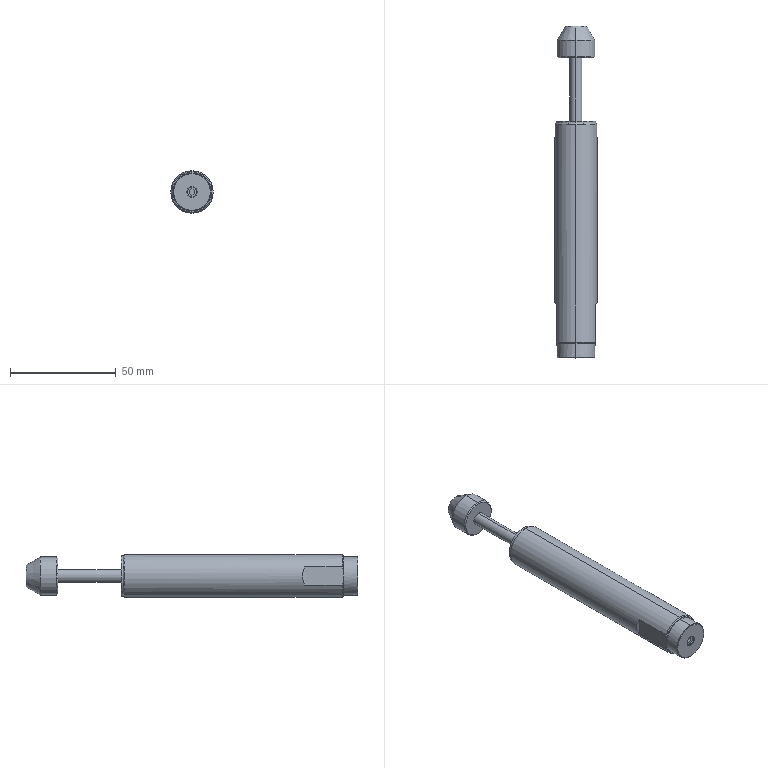Part | SolidWorks | features BaseBody 1 | 1 solid | 46 faces | box 20 x 157 x 20 mm | volume 38514 mm3 | plane 19 | cone 15 | cylinder 12 | commonest cylinder face diameters 18 x4 4.459 x2 6 x2 19 x2 20 x2
STEP:
#1=CARTESIAN_POINT('',(0.,0.2705,2.23));
#2=VERTEX_POINT('',#1);
#3=CARTESIAN_POINT('',(0.,0.2705,-2.23));
#4=VERTEX_POINT('',#3);
#5=CARTESIAN_POINT('',(0.,0.2705,0.));
#6=DIRECTION('',(0.,-1.,0.));
#7=DIRECTION('',(0.,0.,-1.));
#8=AXIS2_PLACEMENT_3D('',#5,#6,#7);
#9=CIRCLE('',#8,2.23);
#10=EDGE_CURVE('',#2,#4,#9,.T.);
#11=ORIENTED_EDGE('',*,*,#10,.F.);
#12=CARTESIAN_POINT('',(0.,0.,2.5));
#13=VERTEX_POINT('',#12);
#14=CARTESIAN_POINT('',(0.,0.2705,2.23));
#15=DIRECTION('',(0.,-0.7071,0.7071));
#16=VECTOR('',#15,1000.);
#17=LINE('',#14,#16);
#18=EDGE_CURVE('',#2,#13,#17,.T.);
#19=ORIENTED_EDGE('',*,*,#18,.T.);
#20=CARTESIAN_POINT('',(0.,0.,-2.5));
#21=VERTEX_POINT('',#20);
#22=CARTESIAN_POINT('',(0.,0.,0.));
#23=DIRECTION('',(0.,-1.,0.));
#24=DIRECTION('',(0.,0.,-1.));
#25=AXIS2_PLACEMENT_3D('',#22,#23,#24);
#26=CIRCLE('',#25,2.5);
#27=EDGE_CURVE('',#13,#21,#26,.T.);
#28=ORIENTED_EDGE('',*,*,#27,.T.);
#29=CARTESIAN_POINT('',(0.,0.2705,-2.23));
#30=DIRECTION('',(0.,-0.7071,-0.7071));
#31=VECTOR('',#30,1000.);
#32=LINE('',#29,#31);
#33=EDGE_CURVE('',#4,#21,#32,.T.);
#34=ORIENTED_EDGE('',*,*,#33,.F.);
#35=EDGE_LOOP('',(#11,#19,#28,#34));
#36=FACE_OUTER_BOUND('',#35,.T.);
#37=CARTESIAN_POINT('',(0.,0.2705,0.));
#38=DIRECTION('',(0.,-1.,0.));
#39=DIRECTION('',(0.,0.,-1.));
#40=AXIS2_PLACEMENT_3D('',#37,#38,#39);
#41=CONICAL_SURFACE('',#40,2.23,0.7854);
#42=ADVANCED_FACE('',(#36),#41,.F.);
#43=CARTESIAN_POINT('',(0.,0.2705,0.));
#44=DIRECTION('',(0.,-1.,0.));
#45=DIRECTION('',(0.,0.,-1.));
#46=AXIS2_PLACEMENT_3D('',#43,#44,#45);
#47=CIRCLE('',#46,2.23);
#48=EDGE_CURVE('',#4,#2,#47,.T.);
#49=ORIENTED_EDGE('',*,*,#48,.T.);
#50=CARTESIAN_POINT('',(0.,0.9295,2.23));
#51=VERTEX_POINT('',#50);
#52=CARTESIAN_POINT('',(0.,0.,2.23));
#53=DIRECTION('',(0.,1.,0.));
#54=VECTOR('',#53,1000.);
#55=LINE('',#52,#54);
#56=EDGE_CURVE('',#2,#51,#55,.T.);
#57=ORIENTED_EDGE('',*,*,#56,.T.);
#58=CARTESIAN_POINT('',(0.,0.9295,-2.23));
#59=VERTEX_POINT('',#58);
#60=CARTESIAN_POINT('',(0.,0.9295,0.));
#61=DIRECTION('',(0.,-1.,0.));
#62=DIRECTION('',(0.,0.,-1.));
#63=AXIS2_PLACEMENT_3D('',#60,#61,#62);
#64=CIRCLE('',#63,2.23);
#65=EDGE_CURVE('',#59,#51,#64,.T.);
#66=ORIENTED_EDGE('',*,*,#65,.F.);
#67=CARTESIAN_POINT('',(0.,0.,-2.23));
#68=DIRECTION('',(0.,1.,0.));
#69=VECTOR('',#68,1000.);
#70=LINE('',#67,#69);
#71=EDGE_CURVE('',#4,#59,#70,.T.);
#72=ORIENTED_EDGE('',*,*,#71,.F.);
#73=EDGE_LOOP('',(#49,#57,#66,#72));
#74=FACE_OUTER_BOUND('',#73,.T.);
#75=CARTESIAN_POINT('',(0.,0.,0.));
#76=DIRECTION('',(0.,1.,0.));
#77=DIRECTION('',(0.,0.,-1.));
#78=AXIS2_PLACEMENT_3D('',#75,#76,#77);
#79=CYLINDRICAL_SURFACE('',#78,2.23);
#80=ADVANCED_FACE('',(#74),#79,.F.);
#81=CARTESIAN_POINT('',(0.,0.9295,0.));
#82=DIRECTION('',(0.,-1.,0.));
#83=DIRECTION('',(0.,0.,-1.));
#84=AXIS2_PLACEMENT_3D('',#81,#82,#83);
#85=CIRCLE('',#84,2.23);
#86=EDGE_CURVE('',#51,#59,#85,.T.);
#87=ORIENTED_EDGE('',*,*,#86,.T.);
#88=CARTESIAN_POINT('',(0.,1.2,-2.5));
#89=VERTEX_POINT('',#88);
#90=CARTESIAN_POINT('',(0.,1.2,-2.5));
#91=DIRECTION('',(0.,0.7071,-0.7071));
#92=VECTOR('',#91,1000.);
#93=LINE('',#90,#92);
#94=EDGE_CURVE('',#59,#89,#93,.T.);
#95=ORIENTED_EDGE('',*,*,#94,.T.);
#96=CARTESIAN_POINT('',(0.,1.2,2.5));
#97=VERTEX_POINT('',#96);
#98=CARTESIAN_POINT('',(0.,1.2,0.));
#99=DIRECTION('',(0.,-1.,0.));
#100=DIRECTION('',(0.,0.,-1.));
#101=AXIS2_PLACEMENT_3D('',#98,#99,#100);
#102=CIRCLE('',#101,2.5);
#103=EDGE_CURVE('',#97,#89,#102,.T.);
#104=ORIENTED_EDGE('',*,*,#103,.F.);
#105=CARTESIAN_POINT('',(0.,1.2,2.5));
#106=DIRECTION('',(0.,0.7071,0.7071));
#107=VECTOR('',#106,1000.);
#108=LINE('',#105,#107);
#109=EDGE_CURVE('',#51,#97,#108,.T.);
#110=ORIENTED_EDGE('',*,*,#109,.F.);
#111=EDGE_LOOP('',(#87,#95,#104,#110));
#112=FACE_OUTER_BOUND('',#111,.T.);
#113=CARTESIAN_POINT('',(0.,1.2,0.));
#114=DIRECTION('',(0.,1.,0.));
#115=DIRECTION('',(0.,0.,1.));
#116=AXIS2_PLACEMENT_3D('',#113,#114,#115);
#117=CONICAL_SURFACE('',#116,2.5,0.7854);
#118=ADVANCED_FACE('',(#112),#117,.F.);
#119=CARTESIAN_POINT('',(0.,0.,-8.7));
#120=VERTEX_POINT('',#119);
#121=CARTESIAN_POINT('',(0.,0.,8.7));
#122=VERTEX_POINT('',#121);
#123=CARTESIAN_POINT('',(0.,0.,0.));
#124=DIRECTION('',(0.,-1.,0.));
#125=DIRECTION('',(0.,0.,-1.));
#126=AXIS2_PLACEMENT_3D('',#123,#124,#125);
#127=CIRCLE('',#126,8.7);
#128=EDGE_CURVE('',#120,#122,#127,.T.);
#129=ORIENTED_EDGE('',*,*,#128,.F.);
#130=CARTESIAN_POINT('',(0.,0.3,-9.));
#131=VERTEX_POINT('',#130);
#132=CARTESIAN_POINT('',(0.,0.3,-9.));
#133=DIRECTION('',(0.,0.7071,-0.7071));
#134=VECTOR('',#133,1000.);
#135=LINE('',#132,#134);
#136=EDGE_CURVE('',#120,#131,#135,.T.);
#137=ORIENTED_EDGE('',*,*,#136,.T.);
#138=CARTESIAN_POINT('',(0.,0.3,9.));
#139=VERTEX_POINT('',#138);
#140=CARTESIAN_POINT('',(0.,0.3,0.));
#141=DIRECTION('',(0.,-1.,0.));
#142=DIRECTION('',(0.,0.,-1.));
#143=AXIS2_PLACEMENT_3D('',#140,#141,#142);
#144=CIRCLE('',#143,9.);
#145=EDGE_CURVE('',#131,#139,#144,.T.);
#146=ORIENTED_EDGE('',*,*,#145,.T.);
#147=CARTESIAN_POINT('',(0.,0.3,9.));
#148=DIRECTION('',(0.,0.7071,0.7071));
#149=VECTOR('',#148,1000.);
#150=LINE('',#147,#149);
#151=EDGE_CURVE('',#122,#139,#150,.T.);
#152=ORIENTED_EDGE('',*,*,#151,.F.);
#153=EDGE_LOOP('',(#129,#137,#146,#152));
#154=FACE_OUTER_BOUND('',#153,.T.);
#155=CARTESIAN_POINT('',(0.,0.3,0.));
#156=DIRECTION('',(0.,1.,0.));
#157=DIRECTION('',(0.,0.,1.));
#158=AXIS2_PLACEMENT_3D('',#155,#156,#157);
#159=CONICAL_SURFACE('',#158,9.,0.7854);
#160=ADVANCED_FACE('',(#154),#159,.T.);
#161=CARTESIAN_POINT('',(0.,0.3,0.));
#162=DIRECTION('',(0.,-1.,0.));
#163=DIRECTION('',(0.,0.,-1.));
#164=AXIS2_PLACEMENT_3D('',#161,#162,#163);
#165=CIRCLE('',#164,9.);
#166=EDGE_CURVE('',#139,#131,#165,.T.);
#167=ORIENTED_EDGE('',*,*,#166,.F.);
#168=CARTESIAN_POINT('',(0.,7.,9.));
#169=VERTEX_POINT('',#168);
#170=CARTESIAN_POINT('',(0.,0.,9.));
#171=DIRECTION('',(0.,1.,0.));
#172=VECTOR('',#171,1000.);
#173=LINE('',#170,#172);
#174=EDGE_CURVE('',#139,#169,#173,.T.);
#175=ORIENTED_EDGE('',*,*,#174,.T.);
#176=CARTESIAN_POINT('',(-9.,7.,0.));
#177=VERTEX_POINT('',#176);
#178=CARTESIAN_POINT('',(0.,7.,0.));
#179=DIRECTION('',(0.,-1.,0.));
#180=DIRECTION('',(0.,0.,-1.));
#181=AXIS2_PLACEMENT_3D('',#178,#179,#180);
#182=CIRCLE('',#181,9.);
#183=EDGE_CURVE('',#169,#177,#182,.T.);
#184=ORIENTED_EDGE('',*,*,#183,.T.);
#185=CARTESIAN_POINT('',(0.,7.,-9.));
#186=VERTEX_POINT('',#185);
#187=CARTESIAN_POINT('',(0.,7.,0.));
#188=DIRECTION('',(0.,-1.,0.));
#189=DIRECTION('',(0.,0.,-1.));
#190=AXIS2_PLACEMENT_3D('',#187,#188,#189);
#191=CIRCLE('',#190,9.);
#192=EDGE_CURVE('',#177,#186,#191,.T.);
#193=ORIENTED_EDGE('',*,*,#192,.T.);
#194=CARTESIAN_POINT('',(0.,0.,-9.));
#195=DIRECTION('',(0.,1.,0.));
#196=VECTOR('',#195,1000.);
#197=LINE('',#194,#196);
#198=EDGE_CURVE('',#131,#186,#197,.T.);
#199=ORIENTED_EDGE('',*,*,#198,.F.);
#200=EDGE_LOOP('',(#167,#175,#184,#193,#199));
#201=FACE_OUTER_BOUND('',#200,.T.);
#202=CARTESIAN_POINT('',(0.,0.,0.));
#203=DIRECTION('',(0.,1.,0.));
#204=DIRECTION('',(0.,0.,-1.));
#205=AXIS2_PLACEMENT_3D('',#202,#203,#204);
#206=CYLINDRICAL_SURFACE('',#205,9.);
#207=ADVANCED_FACE('',(#201),#206,.T.);
#208=CARTESIAN_POINT('',(0.,7.46,10.));
#209=VERTEX_POINT('',#208);
#210=CARTESIAN_POINT('',(-9.,7.46,4.359));
#211=VERTEX_POINT('',#210);
#212=CARTESIAN_POINT('',(0.,7.46,0.));
#213=DIRECTION('',(0.,-1.,0.));
#214=DIRECTION('',(0.,0.,-1.));
#215=AXIS2_PLACEMENT_3D('',#212,#213,#214);
#216=CIRCLE('',#215,10.);
#217=EDGE_CURVE('',#209,#211,#216,.T.);
#218=ORIENTED_EDGE('',*,*,#217,.F.);
#219=CARTESIAN_POINT('',(0.,110.54,10.));
#220=VERTEX_POINT('',#219);
#221=CARTESIAN_POINT('',(0.,0.,10.));
#222=DIRECTION('',(0.,1.,0.));
#223=VECTOR('',#222,1000.);
#224=LINE('',#221,#223);
#225=EDGE_CURVE('',#209,#220,#224,.T.);
#226=ORIENTED_EDGE('',*,*,#225,.T.);
#227=CARTESIAN_POINT('',(0.,110.54,-10.));
#228=VERTEX_POINT('',#227);
#229=CARTESIAN_POINT('',(0.,110.54,0.));
#230=DIRECTION('',(0.,-1.,0.));
#231=DIRECTION('',(0.,0.,-1.));
#232=AXIS2_PLACEMENT_3D('',#229,#230,#231);
#233=CIRCLE('',#232,10.);
#234=EDGE_CURVE('',#220,#228,#233,.T.);
#235=ORIENTED_EDGE('',*,*,#234,.T.);
#236=CARTESIAN_POINT('',(0.,7.46,-10.));
#237=VERTEX_POINT('',#236);
#238=CARTESIAN_POINT('',(0.,0.,-10.));
#239=DIRECTION('',(0.,1.,0.));
#240=VECTOR('',#239,1000.);
#241=LINE('',#238,#240);
#242=EDGE_CURVE('',#237,#228,#241,.T.);
#243=ORIENTED_EDGE('',*,*,#242,.F.);
#244=CARTESIAN_POINT('',(-9.,7.46,-4.359));
#245=VERTEX_POINT('',#244);
#246=CARTESIAN_POINT('',(0.,7.46,0.));
#247=DIRECTION('',(0.,-1.,0.));
#248=DIRECTION('',(0.,0.,-1.));
#249=AXIS2_PLACEMENT_3D('',#246,#247,#248);
#250=CIRCLE('',#249,10.);
#251=EDGE_CURVE('',#245,#237,#250,.T.);
#252=ORIENTED_EDGE('',*,*,#251,.F.);
#253=CARTESIAN_POINT('',(-9.,25.177,-4.359));
#254=VERTEX_POINT('',#253);
#255=CARTESIAN_POINT('',(-9.,0.,-4.359));
#256=DIRECTION('',(0.,-1.,0.));
#257=VECTOR('',#256,1000.);
#258=LINE('',#255,#257);
#259=EDGE_CURVE('',#254,#245,#258,.T.);
#260=ORIENTED_EDGE('',*,*,#259,.F.);
#261=CARTESIAN_POINT('',(-9.,25.177,4.359));
#262=VERTEX_POINT('',#261);
#263=CARTESIAN_POINT('',(-9.,25.177,4.359));
#264=CARTESIAN_POINT('',(-10.357,26.534,1.557));
#265=CARTESIAN_POINT('',(-10.357,26.534,-1.557));
#266=CARTESIAN_POINT('',(-9.,25.177,-4.359));
#267=(BOUNDED_CURVE()B_SPLINE_CURVE(3,(#263,#264,#265,#266),.UNSPECIFIED.,.F.,.T.)B_SPLINE_CURVE_WITH_KNOTS((4,4),(2.691,3.593),.UNSPECIFIED.)CURVE()GEOMETRIC_REPRESENTATION_ITEM()RATIONAL_B_SPLINE_CURVE((1.,0.9333,0.9333,1.))REPRESENTATION_ITEM(''));
#268=EDGE_CURVE('',#262,#254,#267,.T.);
#269=ORIENTED_EDGE('',*,*,#268,.F.);
#270=CARTESIAN_POINT('',(-9.,0.,4.359));
#271=DIRECTION('',(0.,1.,0.));
#272=VECTOR('',#271,1000.);
#273=LINE('',#270,#272);
#274=EDGE_CURVE('',#211,#262,#273,.T.);
#275=ORIENTED_EDGE('',*,*,#274,.F.);
#276=EDGE_LOOP('',(#218,#226,#235,#243,#252,#260,#269,#275));
#277=FACE_OUTER_BOUND('',#276,.T.);
#278=CARTESIAN_POINT('',(0.,0.,0.));
#279=DIRECTION('',(0.,1.,0.));
#280=DIRECTION('',(0.,0.,-1.));
#281=AXIS2_PLACEMENT_3D('',#278,#279,#280);
#282=CYLINDRICAL_SURFACE('',#281,10.);
#283=ADVANCED_FACE('',(#277),#282,.T.);
#284=CARTESIAN_POINT('',(0.,7.,9.54));
#285=VERTEX_POINT('',#284);
#286=CARTESIAN_POINT('',(-9.,7.,3.164));
#287=VERTEX_POINT('',#286);
#288=CARTESIAN_POINT('',(0.,7.,0.));
#289=DIRECTION('',(0.,-1.,0.));
#290=DIRECTION('',(0.,0.,-1.));
#291=AXIS2_PLACEMENT_3D('',#288,#289,#290);
#292=CIRCLE('',#291,9.54);
#293=EDGE_CURVE('',#285,#287,#292,.T.);
#294=ORIENTED_EDGE('',*,*,#293,.F.);
#295=CARTESIAN_POINT('',(0.,7.46,10.));
#296=DIRECTION('',(0.,0.7071,0.7071));
#297=VECTOR('',#296,1000.);
#298=LINE('',#295,#297);
#299=EDGE_CURVE('',#285,#209,#298,.T.);
#300=ORIENTED_EDGE('',*,*,#299,.T.);
#301=ORIENTED_EDGE('',*,*,#217,.T.);
#302=CARTESIAN_POINT('',(-9.,7.,3.164));
#303=CARTESIAN_POINT('',(-9.,7.134,3.57));
#304=CARTESIAN_POINT('',(-9.,7.289,3.967));
#305=CARTESIAN_POINT('',(-9.,7.46,4.359));
#306=B_SPLINE_CURVE_WITH_KNOTS('',3,(#302,#303,#304,#305),.UNSPECIFIED.,.F.,.F.,(4,4),(0.,0.00128),.UNSPECIFIED.);
#307=EDGE_CURVE('',#287,#211,#306,.T.);
#308=ORIENTED_EDGE('',*,*,#307,.F.);
#309=EDGE_LOOP('',(#294,#300,#301,#308));
#310=FACE_OUTER_BOUND('',#309,.T.);
#311=CARTESIAN_POINT('',(0.,7.46,0.));
#312=DIRECTION('',(0.,1.,0.));
#313=DIRECTION('',(0.,0.,1.));
#314=AXIS2_PLACEMENT_3D('',#311,#312,#313);
#315=CONICAL_SURFACE('',#314,10.,0.7854);
#316=ADVANCED_FACE('',(#310),#315,.T.);
#317=CARTESIAN_POINT('',(0.,111.,-9.54));
#318=VERTEX_POINT('',#317);
#319=CARTESIAN_POINT('',(0.,111.,9.54));
#320=VERTEX_POINT('',#319);
#321=CARTESIAN_POINT('',(0.,111.,0.));
#322=DIRECTION('',(0.,-1.,0.));
#323=DIRECTION('',(0.,0.,-1.));
#324=AXIS2_PLACEMENT_3D('',#321,#322,#323);
#325=CIRCLE('',#324,9.54);
#326=EDGE_CURVE('',#318,#320,#325,.T.);
#327=ORIENTED_EDGE('',*,*,#326,.T.);
#328=CARTESIAN_POINT('',(0.,111.,9.54));
#329=DIRECTION('',(0.,-0.7071,0.7071));
#330=VECTOR('',#329,1000.);
#331=LINE('',#328,#330);
#332=EDGE_CURVE('',#320,#220,#331,.T.);
#333=ORIENTED_EDGE('',*,*,#332,.T.);
#334=CARTESIAN_POINT('',(0.,110.54,0.));
#335=DIRECTION('',(0.,-1.,0.));
#336=DIRECTION('',(0.,0.,-1.));
#337=AXIS2_PLACEMENT_3D('',#334,#335,#336);
#338=CIRCLE('',#337,10.);
#339=EDGE_CURVE('',#228,#220,#338,.T.);
#340=ORIENTED_EDGE('',*,*,#339,.F.);
#341=CARTESIAN_POINT('',(0.,111.,-9.54));
#342=DIRECTION('',(0.,-0.7071,-0.7071));
#343=VECTOR('',#342,1000.);
#344=LINE('',#341,#343);
#345=EDGE_CURVE('',#318,#228,#344,.T.);
#346=ORIENTED_EDGE('',*,*,#345,.F.);
#347=EDGE_LOOP('',(#327,#333,#340,#346));
#348=FACE_OUTER_BOUND('',#347,.T.);
#349=CARTESIAN_POINT('',(0.,111.,0.));
#350=DIRECTION('',(0.,-1.,0.));
#351=DIRECTION('',(0.,0.,-1.));
#352=AXIS2_PLACEMENT_3D('',#349,#350,#351);
#353=CONICAL_SURFACE('',#352,9.54,0.7854);
#354=ADVANCED_FACE('',(#348),#353,.T.);
#355=CARTESIAN_POINT('',(0.,111.,9.5));
#356=VERTEX_POINT('',#355);
#357=CARTESIAN_POINT('',(0.,111.,-9.5));
#358=VERTEX_POINT('',#357);
#359=CARTESIAN_POINT('',(0.,111.,0.));
#360=DIRECTION('',(0.,-1.,0.));
#361=DIRECTION('',(0.,0.,-1.));
#362=AXIS2_PLACEMENT_3D('',#359,#360,#361);
#363=CIRCLE('',#362,9.5);
#364=EDGE_CURVE('',#356,#358,#363,.T.);
#365=ORIENTED_EDGE('',*,*,#364,.F.);
#366=CARTESIAN_POINT('',(0.,112.,9.5));
#367=VERTEX_POINT('',#366);
#368=CARTESIAN_POINT('',(0.,0.,9.5));
#369=DIRECTION('',(0.,1.,0.));
#370=VECTOR('',#369,1000.);
#371=LINE('',#368,#370);
#372=EDGE_CURVE('',#356,#367,#371,.T.);
#373=ORIENTED_EDGE('',*,*,#372,.T.);
#374=CARTESIAN_POINT('',(0.,112.,-9.5));
#375=VERTEX_POINT('',#374);
#376=CARTESIAN_POINT('',(0.,112.,0.));
#377=DIRECTION('',(0.,-1.,0.));
#378=DIRECTION('',(0.,0.,-1.));
#379=AXIS2_PLACEMENT_3D('',#376,#377,#378);
#380=CIRCLE('',#379,9.5);
#381=EDGE_CURVE('',#367,#375,#380,.T.);
#382=ORIENTED_EDGE('',*,*,#381,.T.);
#383=CARTESIAN_POINT('',(0.,0.,-9.5));
#384=DIRECTION('',(0.,1.,0.));
#385=VECTOR('',#384,1000.);
#386=LINE('',#383,#385);
#387=EDGE_CURVE('',#358,#375,#386,.T.);
#388=ORIENTED_EDGE('',*,*,#387,.F.);
#389=EDGE_LOOP('',(#365,#373,#382,#388));
#390=FACE_OUTER_BOUND('',#389,.T.);
#391=CARTESIAN_POINT('',(0.,0.,0.));
#392=DIRECTION('',(0.,1.,0.));
#393=DIRECTION('',(0.,0.,-1.));
#394=AXIS2_PLACEMENT_3D('',#391,#392,#393);
#395=CYLINDRICAL_SURFACE('',#394,9.5);
#396=ADVANCED_FACE('',(#390),#395,.T.);
#397=CARTESIAN_POINT('',(0.,112.,3.));
#398=VERTEX_POINT('',#397);
#399=CARTESIAN_POINT('',(0.,112.,-3.));
#400=VERTEX_POINT('',#399);
#401=CARTESIAN_POINT('',(0.,112.,0.));
#402=DIRECTION('',(0.,-1.,0.));
#403=DIRECTION('',(0.,0.,-1.));
#404=AXIS2_PLACEMENT_3D('',#401,#402,#403);
#405=CIRCLE('',#404,3.);
#406=EDGE_CURVE('',#398,#400,#405,.T.);
#407=ORIENTED_EDGE('',*,*,#406,.F.);
#408=CARTESIAN_POINT('',(0.,142.,3.));
#409=VERTEX_POINT('',#408);
#410=CARTESIAN_POINT('',(0.,0.,3.));
#411=DIRECTION('',(0.,1.,0.));
#412=VECTOR('',#411,1000.);
#413=LINE('',#410,#412);
#414=EDGE_CURVE('',#398,#409,#413,.T.);
#415=ORIENTED_EDGE('',*,*,#414,.T.);
#416=CARTESIAN_POINT('',(0.,142.,-3.));
#417=VERTEX_POINT('',#416);
#418=CARTESIAN_POINT('',(0.,142.,0.));
#419=DIRECTION('',(0.,-1.,0.));
#420=DIRECTION('',(0.,0.,-1.));
#421=AXIS2_PLACEMENT_3D('',#418,#419,#420);
#422=CIRCLE('',#421,3.);
#423=EDGE_CURVE('',#409,#417,#422,.T.);
#424=ORIENTED_EDGE('',*,*,#423,.T.);
#425=CARTESIAN_POINT('',(0.,0.,-3.));
#426=DIRECTION('',(0.,1.,0.));
#427=VECTOR('',#426,1000.);
#428=LINE('',#425,#427);
#429=EDGE_CURVE('',#400,#417,#428,.T.);
#430=ORIENTED_EDGE('',*,*,#429,.F.);
#431=EDGE_LOOP('',(#407,#415,#424,#430));
#432=FACE_OUTER_BOUND('',#431,.T.);
#433=CARTESIAN_POINT('',(0.,0.,0.));
#434=DIRECTION('',(0.,1.,0.));
#435=DIRECTION('',(0.,0.,-1.));
#436=AXIS2_PLACEMENT_3D('',#433,#434,#435);
#437=CYLINDRICAL_SURFACE('',#436,3.);
#438=ADVANCED_FACE('',(#432),#437,.T.);
#439=CARTESIAN_POINT('',(0.,142.,-8.5));
#440=VERTEX_POINT('',#439);
#441=CARTESIAN_POINT('',(0.,142.,8.5));
#442=VERTEX_POINT('',#441);
#443=CARTESIAN_POINT('',(0.,142.,0.));
#444=DIRECTION('',(0.,-1.,0.));
#445=DIRECTION('',(0.,0.,-1.));
#446=AXIS2_PLACEMENT_3D('',#443,#444,#445);
#447=CIRCLE('',#446,8.5);
#448=EDGE_CURVE('',#440,#442,#447,.T.);
#449=ORIENTED_EDGE('',*,*,#448,.F.);
#450=CARTESIAN_POINT('',(0.,142.5,-9.));
#451=VERTEX_POINT('',#450);
#452=CARTESIAN_POINT('',(0.,142.5,-9.));
#453=DIRECTION('',(0.,0.7071,-0.7071));
#454=VECTOR('',#453,1000.);
#455=LINE('',#452,#454);
#456=EDGE_CURVE('',#440,#451,#455,.T.);
#457=ORIENTED_EDGE('',*,*,#456,.T.);
#458=CARTESIAN_POINT('',(0.,142.5,9.));
#459=VERTEX_POINT('',#458);
#460=CARTESIAN_POINT('',(0.,142.5,0.));
#461=DIRECTION('',(0.,-1.,0.));
#462=DIRECTION('',(0.,0.,-1.));
#463=AXIS2_PLACEMENT_3D('',#460,#461,#462);
#464=CIRCLE('',#463,9.);
#465=EDGE_CURVE('',#451,#459,#464,.T.);
#466=ORIENTED_EDGE('',*,*,#465,.T.);
#467=CARTESIAN_POINT('',(0.,142.5,9.));
#468=DIRECTION('',(0.,0.7071,0.7071));
#469=VECTOR('',#468,1000.);
#470=LINE('',#467,#469);
#471=EDGE_CURVE('',#442,#459,#470,.T.);
#472=ORIENTED_EDGE('',*,*,#471,.F.);
#473=EDGE_LOOP('',(#449,#457,#466,#472));
#474=FACE_OUTER_BOUND('',#473,.T.);
#475=CARTESIAN_POINT('',(0.,142.5,0.));
#476=DIRECTION('',(0.,1.,0.));
#477=DIRECTION('',(0.,0.,1.));
#478=AXIS2_PLACEMENT_3D('',#475,#476,#477);
#479=CONICAL_SURFACE('',#478,9.,0.7854);
#480=ADVANCED_FACE('',(#474),#479,.T.);
#481=CARTESIAN_POINT('',(0.,142.5,0.));
#482=DIRECTION('',(0.,-1.,0.));
#483=DIRECTION('',(0.,0.,-1.));
#484=AXIS2_PLACEMENT_3D('',#481,#482,#483);
#485=CIRCLE('',#484,9.);
#486=EDGE_CURVE('',#459,#451,#485,.T.);
#487=ORIENTED_EDGE('',*,*,#486,.F.);
#488=CARTESIAN_POINT('',(0.,150.333,9.));
#489=VERTEX_POINT('',#488);
#490=CARTESIAN_POINT('',(0.,0.,9.));
#491=DIRECTION('',(0.,1.,0.));
#492=VECTOR('',#491,1000.);
#493=LINE('',#490,#492);
#494=EDGE_CURVE('',#459,#489,#493,.T.);
#495=ORIENTED_EDGE('',*,*,#494,.T.);
#496=CARTESIAN_POINT('',(0.,150.333,-9.));
#497=VERTEX_POINT('',#496);
#498=CARTESIAN_POINT('',(0.,150.333,0.));
#499=DIRECTION('',(0.,-1.,0.));
#500=DIRECTION('',(0.,0.,-1.));
#501=AXIS2_PLACEMENT_3D('',#498,#499,#500);
#502=CIRCLE('',#501,9.);
#503=EDGE_CURVE('',#489,#497,#502,.T.);
#504=ORIENTED_EDGE('',*,*,#503,.T.);
#505=CARTESIAN_POINT('',(0.,0.,-9.));
#506=DIRECTION('',(0.,1.,0.));
#507=VECTOR('',#506,1000.);
#508=LINE('',#505,#507);
#509=EDGE_CURVE('',#451,#497,#508,.T.);
#510=ORIENTED_EDGE('',*,*,#509,.F.);
#511=EDGE_LOOP('',(#487,#495,#504,#510));
#512=FACE_OUTER_BOUND('',#511,.T.);
#513=CARTESIAN_POINT('',(0.,0.,0.));
#514=DIRECTION('',(0.,1.,0.));
#515=DIRECTION('',(0.,0.,-1.));
#516=AXIS2_PLACEMENT_3D('',#513,#514,#515);
#517=CYLINDRICAL_SURFACE('',#516,9.);
#518=ADVANCED_FACE('',(#512),#517,.T.);
#519=CARTESIAN_POINT('',(0.,157.,-5.151));
#520=VERTEX_POINT('',#519);
#521=CARTESIAN_POINT('',(0.,157.,5.151));
#522=VERTEX_POINT('',#521);
#523=CARTESIAN_POINT('',(0.,157.,0.));
#524=DIRECTION('',(0.,-1.,0.));
#525=DIRECTION('',(0.,0.,-1.));
#526=AXIS2_PLACEMENT_3D('',#523,#524,#525);
#527=CIRCLE('',#526,5.151);
#528=EDGE_CURVE('',#520,#522,#527,.T.);
#529=ORIENTED_EDGE('',*,*,#528,.T.);
#530=CARTESIAN_POINT('',(0.,157.,5.151));
#531=DIRECTION('',(0.,-0.866,0.5));
#532=VECTOR('',#531,1000.);
#533=LINE('',#530,#532);
#534=EDGE_CURVE('',#522,#489,#533,.T.);
#535=ORIENTED_EDGE('',*,*,#534,.T.);
#536=CARTESIAN_POINT('',(0.,150.333,0.));
#537=DIRECTION('',(0.,-1.,0.));
#538=DIRECTION('',(0.,0.,-1.));
#539=AXIS2_PLACEMENT_3D('',#536,#537,#538);
#540=CIRCLE('',#539,9.);
#541=EDGE_CURVE('',#497,#489,#540,.T.);
#542=ORIENTED_EDGE('',*,*,#541,.F.);
#543=CARTESIAN_POINT('',(0.,157.,-5.151));
#544=DIRECTION('',(0.,-0.866,-0.5));
#545=VECTOR('',#544,1000.);
#546=LINE('',#543,#545);
#547=EDGE_CURVE('',#520,#497,#546,.T.);
#548=ORIENTED_EDGE('',*,*,#547,.F.);
#549=EDGE_LOOP('',(#529,#535,#542,#548));
#550=FACE_OUTER_BOUND('',#549,.T.);
#551=CARTESIAN_POINT('',(0.,157.,0.));
#552=DIRECTION('',(0.,-1.,0.));
#553=DIRECTION('',(0.,0.,-1.));
#554=AXIS2_PLACEMENT_3D('',#551,#552,#553);
#555=CONICAL_SURFACE('',#554,5.151,0.5236);
#556=ADVANCED_FACE('',(#550),#555,.T.);
#557=ORIENTED_EDGE('',*,*,#259,.T.);
#558=CARTESIAN_POINT('',(-9.,7.,-3.164));
#559=VERTEX_POINT('',#558);
#560=CARTESIAN_POINT('',(-9.,7.46,-4.359));
#561=CARTESIAN_POINT('',(-9.,7.289,-3.967));
#562=CARTESIAN_POINT('',(-9.,7.134,-3.57));
#563=CARTESIAN_POINT('',(-9.,7.,-3.164));
#564=B_SPLINE_CURVE_WITH_KNOTS('',3,(#560,#561,#562,#563),.UNSPECIFIED.,.F.,.F.,(4,4),(0.,0.00128),.UNSPECIFIED.);
#565=EDGE_CURVE('',#245,#559,#564,.T.);
#566=ORIENTED_EDGE('',*,*,#565,.T.);
#567=CARTESIAN_POINT('',(-9.,7.,0.));
#568=DIRECTION('',(0.,0.,1.));
#569=VECTOR('',#568,1000.);
#570=LINE('',#567,#569);
#571=EDGE_CURVE('',#559,#177,#570,.T.);
#572=ORIENTED_EDGE('',*,*,#571,.T.);
#573=CARTESIAN_POINT('',(-9.,7.,0.));
#574=DIRECTION('',(0.,0.,1.));
#575=VECTOR('',#574,1000.);
#576=LINE('',#573,#575);
#577=EDGE_CURVE('',#177,#287,#576,.T.);
#578=ORIENTED_EDGE('',*,*,#577,.T.);
#579=ORIENTED_EDGE('',*,*,#307,.T.);
#580=ORIENTED_EDGE('',*,*,#274,.T.);
#581=CARTESIAN_POINT('',(-9.,25.177,20.));
#582=DIRECTION('',(0.,0.,-1.));
#583=VECTOR('',#582,1000.);
#584=LINE('',#581,#583);
#585=EDGE_CURVE('',#262,#254,#584,.T.);
#586=ORIENTED_EDGE('',*,*,#585,.T.);
#587=EDGE_LOOP('',(#557,#566,#572,#578,#579,#580,#586));
#588=FACE_OUTER_BOUND('',#587,.T.);
#589=CARTESIAN_POINT('',(-9.,0.,20.));
#590=DIRECTION('',(-1.,0.,0.));
#591=DIRECTION('',(0.,1.,0.));
#592=AXIS2_PLACEMENT_3D('',#589,#590,#591);
#593=PLANE('',#592);
#594=ADVANCED_FACE('',(#588),#593,.T.);
#595=ORIENTED_EDGE('',*,*,#528,.F.);
#596=CARTESIAN_POINT('',(0.,157.,0.));
#597=DIRECTION('',(0.,-1.,0.));
#598=DIRECTION('',(0.,0.,-1.));
#599=AXIS2_PLACEMENT_3D('',#596,#597,#598);
#600=CIRCLE('',#599,5.151);
#601=EDGE_CURVE('',#522,#520,#600,.T.);
#602=ORIENTED_EDGE('',*,*,#601,.F.);
#603=EDGE_LOOP('',(#595,#602));
#604=FACE_OUTER_BOUND('',#603,.T.);
#605=CARTESIAN_POINT('',(0.,157.,0.));
#606=DIRECTION('',(0.,-1.,0.));
#607=DIRECTION('',(0.,0.,-1.));
#608=AXIS2_PLACEMENT_3D('',#605,#606,#607);
#609=PLANE('',#608);
#610=ADVANCED_FACE('',(#604),#609,.F.);
#611=ORIENTED_EDGE('',*,*,#534,.F.);
#612=ORIENTED_EDGE('',*,*,#601,.T.);
#613=ORIENTED_EDGE('',*,*,#547,.T.);
#614=ORIENTED_EDGE('',*,*,#503,.F.);
#615=EDGE_LOOP('',(#611,#612,#613,#614));
#616=FACE_OUTER_BOUND('',#615,.T.);
#617=CARTESIAN_POINT('',(0.,157.,0.));
#618=DIRECTION('',(0.,-1.,0.));
#619=DIRECTION('',(0.,0.,-1.));
#620=AXIS2_PLACEMENT_3D('',#617,#618,#619);
#621=CONICAL_SURFACE('',#620,5.151,0.5236);
#622=ADVANCED_FACE('',(#616),#621,.T.);
#623=ORIENTED_EDGE('',*,*,#494,.F.);
#624=ORIENTED_EDGE('',*,*,#465,.F.);
#625=ORIENTED_EDGE('',*,*,#509,.T.);
#626=ORIENTED_EDGE('',*,*,#541,.T.);
#627=EDGE_LOOP('',(#623,#624,#625,#626));
#628=FACE_OUTER_BOUND('',#627,.T.);
#629=CARTESIAN_POINT('',(0.,0.,0.));
#630=DIRECTION('',(0.,1.,0.));
#631=DIRECTION('',(0.,0.,-1.));
#632=AXIS2_PLACEMENT_3D('',#629,#630,#631);
#633=CYLINDRICAL_SURFACE('',#632,9.);
#634=ADVANCED_FACE('',(#628),#633,.T.);
#635=ORIENTED_EDGE('',*,*,#456,.F.);
#636=CARTESIAN_POINT('',(0.,142.,0.));
#637=DIRECTION('',(0.,-1.,0.));
#638=DIRECTION('',(0.,0.,-1.));
#639=AXIS2_PLACEMENT_3D('',#636,#637,#638);
#640=CIRCLE('',#639,8.5);
#641=EDGE_CURVE('',#442,#440,#640,.T.);
#642=ORIENTED_EDGE('',*,*,#641,.F.);
#643=ORIENTED_EDGE('',*,*,#471,.T.);
#644=ORIENTED_EDGE('',*,*,#486,.T.);
#645=EDGE_LOOP('',(#635,#642,#643,#644));
#646=FACE_OUTER_BOUND('',#645,.T.);
#647=CARTESIAN_POINT('',(0.,142.5,0.));
#648=DIRECTION('',(0.,1.,0.));
#649=DIRECTION('',(0.,0.,1.));
#650=AXIS2_PLACEMENT_3D('',#647,#648,#649);
#651=CONICAL_SURFACE('',#650,9.,0.7854);
#652=ADVANCED_FACE('',(#646),#651,.T.);
#653=CARTESIAN_POINT('',(0.,142.,0.));
#654=DIRECTION('',(0.,-1.,0.));
#655=DIRECTION('',(0.,0.,-1.));
#656=AXIS2_PLACEMENT_3D('',#653,#654,#655);
#657=CIRCLE('',#656,3.);
#658=EDGE_CURVE('',#417,#409,#657,.T.);
#659=ORIENTED_EDGE('',*,*,#658,.F.);
#660=ORIENTED_EDGE('',*,*,#423,.F.);
#661=EDGE_LOOP('',(#659,#660));
#662=FACE_BOUND('',#661,.T.);
#663=ORIENTED_EDGE('',*,*,#641,.T.);
#664=ORIENTED_EDGE('',*,*,#448,.T.);
#665=EDGE_LOOP('',(#663,#664));
#666=FACE_OUTER_BOUND('',#665,.T.);
#667=CARTESIAN_POINT('',(8.5,142.,0.));
#668=DIRECTION('',(0.,1.,0.));
#669=DIRECTION('',(1.,0.,0.));
#670=AXIS2_PLACEMENT_3D('',#667,#668,#669);
#671=PLANE('',#670);
#672=ADVANCED_FACE('',(#662,#666),#671,.F.);
#673=ORIENTED_EDGE('',*,*,#414,.F.);
#674=CARTESIAN_POINT('',(0.,112.,0.));
#675=DIRECTION('',(0.,-1.,0.));
#676=DIRECTION('',(0.,0.,-1.));
#677=AXIS2_PLACEMENT_3D('',#674,#675,#676);
#678=CIRCLE('',#677,3.);
#679=EDGE_CURVE('',#400,#398,#678,.T.);
#680=ORIENTED_EDGE('',*,*,#679,.F.);
#681=ORIENTED_EDGE('',*,*,#429,.T.);
#682=ORIENTED_EDGE('',*,*,#658,.T.);
#683=EDGE_LOOP('',(#673,#680,#681,#682));
#684=FACE_OUTER_BOUND('',#683,.T.);
#685=CARTESIAN_POINT('',(0.,0.,0.));
#686=DIRECTION('',(0.,1.,0.));
#687=DIRECTION('',(0.,0.,-1.));
#688=AXIS2_PLACEMENT_3D('',#685,#686,#687);
#689=CYLINDRICAL_SURFACE('',#688,3.);
#690=ADVANCED_FACE('',(#684),#689,.T.);
#691=ORIENTED_EDGE('',*,*,#679,.T.);
#692=ORIENTED_EDGE('',*,*,#406,.T.);
#693=EDGE_LOOP('',(#691,#692));
#694=FACE_BOUND('',#693,.T.);
#695=CARTESIAN_POINT('',(0.,112.,0.));
#696=DIRECTION('',(0.,-1.,0.));
#697=DIRECTION('',(0.,0.,-1.));
#698=AXIS2_PLACEMENT_3D('',#695,#696,#697);
#699=CIRCLE('',#698,9.5);
#700=EDGE_CURVE('',#375,#367,#699,.T.);
#701=ORIENTED_EDGE('',*,*,#700,.F.);
#702=ORIENTED_EDGE('',*,*,#381,.F.);
#703=EDGE_LOOP('',(#701,#702));
#704=FACE_OUTER_BOUND('',#703,.T.);
#705=CARTESIAN_POINT('',(3.,112.,0.));
#706=DIRECTION('',(0.,-1.,0.));
#707=DIRECTION('',(0.,0.,-1.));
#708=AXIS2_PLACEMENT_3D('',#705,#706,#707);
#709=PLANE('',#708);
#710=ADVANCED_FACE('',(#694,#704),#709,.F.);
#711=ORIENTED_EDGE('',*,*,#372,.F.);
#712=CARTESIAN_POINT('',(0.,111.,0.));
#713=DIRECTION('',(0.,-1.,0.));
#714=DIRECTION('',(0.,0.,-1.));
#715=AXIS2_PLACEMENT_3D('',#712,#713,#714);
#716=CIRCLE('',#715,9.5);
#717=EDGE_CURVE('',#358,#356,#716,.T.);
#718=ORIENTED_EDGE('',*,*,#717,.F.);
#719=ORIENTED_EDGE('',*,*,#387,.T.);
#720=ORIENTED_EDGE('',*,*,#700,.T.);
#721=EDGE_LOOP('',(#711,#718,#719,#720));
#722=FACE_OUTER_BOUND('',#721,.T.);
#723=CARTESIAN_POINT('',(0.,0.,0.));
#724=DIRECTION('',(0.,1.,0.));
#725=DIRECTION('',(0.,0.,-1.));
#726=AXIS2_PLACEMENT_3D('',#723,#724,#725);
#727=CYLINDRICAL_SURFACE('',#726,9.5);
#728=ADVANCED_FACE('',(#722),#727,.T.);
#729=ORIENTED_EDGE('',*,*,#717,.T.);
#730=ORIENTED_EDGE('',*,*,#364,.T.);
#731=EDGE_LOOP('',(#729,#730));
#732=FACE_BOUND('',#731,.T.);
#733=ORIENTED_EDGE('',*,*,#326,.F.);
#734=CARTESIAN_POINT('',(0.,111.,0.));
#735=DIRECTION('',(0.,-1.,0.));
#736=DIRECTION('',(0.,0.,-1.));
#737=AXIS2_PLACEMENT_3D('',#734,#735,#736);
#738=CIRCLE('',#737,9.54);
#739=EDGE_CURVE('',#320,#318,#738,.T.);
#740=ORIENTED_EDGE('',*,*,#739,.F.);
#741=EDGE_LOOP('',(#733,#740));
#742=FACE_OUTER_BOUND('',#741,.T.);
#743=CARTESIAN_POINT('',(9.5,111.,0.));
#744=DIRECTION('',(0.,-1.,0.));
#745=DIRECTION('',(0.,0.,-1.));
#746=AXIS2_PLACEMENT_3D('',#743,#744,#745);
#747=PLANE('',#746);
#748=ADVANCED_FACE('',(#732,#742),#747,.F.);
#749=ORIENTED_EDGE('',*,*,#332,.F.);
#750=ORIENTED_EDGE('',*,*,#739,.T.);
#751=ORIENTED_EDGE('',*,*,#345,.T.);
#752=ORIENTED_EDGE('',*,*,#234,.F.);
#753=EDGE_LOOP('',(#749,#750,#751,#752));
#754=FACE_OUTER_BOUND('',#753,.T.);
#755=CARTESIAN_POINT('',(0.,111.,0.));
#756=DIRECTION('',(0.,-1.,0.));
#757=DIRECTION('',(0.,0.,-1.));
#758=AXIS2_PLACEMENT_3D('',#755,#756,#757);
#759=CONICAL_SURFACE('',#758,9.54,0.7854);
#760=ADVANCED_FACE('',(#754),#759,.T.);
#761=ORIENTED_EDGE('',*,*,#299,.F.);
#762=CARTESIAN_POINT('',(9.,7.,3.164));
#763=VERTEX_POINT('',#762);
#764=CARTESIAN_POINT('',(0.,7.,0.));
#765=DIRECTION('',(0.,-1.,0.));
#766=DIRECTION('',(0.,0.,-1.));
#767=AXIS2_PLACEMENT_3D('',#764,#765,#766);
#768=CIRCLE('',#767,9.54);
#769=EDGE_CURVE('',#763,#285,#768,.T.);
#770=ORIENTED_EDGE('',*,*,#769,.F.);
#771=CARTESIAN_POINT('',(9.,7.46,4.359));
#772=VERTEX_POINT('',#771);
#773=CARTESIAN_POINT('',(9.,7.46,4.359));
#774=CARTESIAN_POINT('',(9.,7.289,3.967));
#775=CARTESIAN_POINT('',(9.,7.134,3.57));
#776=CARTESIAN_POINT('',(9.,7.,3.164));
#777=B_SPLINE_CURVE_WITH_KNOTS('',3,(#773,#774,#775,#776),.UNSPECIFIED.,.F.,.F.,(4,4),(0.,0.00128),.UNSPECIFIED.);
#778=EDGE_CURVE('',#772,#763,#777,.T.);
#779=ORIENTED_EDGE('',*,*,#778,.F.);
#780=CARTESIAN_POINT('',(0.,7.46,0.));
#781=DIRECTION('',(0.,-1.,0.));
#782=DIRECTION('',(0.,0.,-1.));
#783=AXIS2_PLACEMENT_3D('',#780,#781,#782);
#784=CIRCLE('',#783,10.);
#785=EDGE_CURVE('',#772,#209,#784,.T.);
#786=ORIENTED_EDGE('',*,*,#785,.T.);
#787=EDGE_LOOP('',(#761,#770,#779,#786));
#788=FACE_OUTER_BOUND('',#787,.T.);
#789=CARTESIAN_POINT('',(0.,7.46,0.));
#790=DIRECTION('',(0.,1.,0.));
#791=DIRECTION('',(0.,0.,1.));
#792=AXIS2_PLACEMENT_3D('',#789,#790,#791);
#793=CONICAL_SURFACE('',#792,10.,0.7854);
#794=ADVANCED_FACE('',(#788),#793,.T.);
#795=ORIENTED_EDGE('',*,*,#225,.F.);
#796=ORIENTED_EDGE('',*,*,#785,.F.);
#797=CARTESIAN_POINT('',(9.,25.177,4.359));
#798=VERTEX_POINT('',#797);
#799=CARTESIAN_POINT('',(9.,0.,4.359));
#800=DIRECTION('',(0.,-1.,0.));
#801=VECTOR('',#800,1000.);
#802=LINE('',#799,#801);
#803=EDGE_CURVE('',#798,#772,#802,.T.);
#804=ORIENTED_EDGE('',*,*,#803,.F.);
#805=CARTESIAN_POINT('',(9.,25.177,-4.359));
#806=VERTEX_POINT('',#805);
#807=CARTESIAN_POINT('',(9.,25.177,-4.359));
#808=CARTESIAN_POINT('',(10.357,26.534,-1.557));
#809=CARTESIAN_POINT('',(10.357,26.534,1.557));
#810=CARTESIAN_POINT('',(9.,25.177,4.359));
#811=(BOUNDED_CURVE()B_SPLINE_CURVE(3,(#807,#808,#809,#810),.UNSPECIFIED.,.F.,.F.)B_SPLINE_CURVE_WITH_KNOTS((4,4),(2.691,3.593),.UNSPECIFIED.)CURVE()GEOMETRIC_REPRESENTATION_ITEM()RATIONAL_B_SPLINE_CURVE((1.,0.9333,0.9333,1.))REPRESENTATION_ITEM(''));
#812=EDGE_CURVE('',#806,#798,#811,.T.);
#813=ORIENTED_EDGE('',*,*,#812,.F.);
#814=CARTESIAN_POINT('',(9.,7.46,-4.359));
#815=VERTEX_POINT('',#814);
#816=CARTESIAN_POINT('',(9.,0.,-4.359));
#817=DIRECTION('',(0.,1.,0.));
#818=VECTOR('',#817,1000.);
#819=LINE('',#816,#818);
#820=EDGE_CURVE('',#815,#806,#819,.T.);
#821=ORIENTED_EDGE('',*,*,#820,.F.);
#822=CARTESIAN_POINT('',(0.,7.46,0.));
#823=DIRECTION('',(0.,-1.,0.));
#824=DIRECTION('',(0.,0.,-1.));
#825=AXIS2_PLACEMENT_3D('',#822,#823,#824);
#826=CIRCLE('',#825,10.);
#827=EDGE_CURVE('',#237,#815,#826,.T.);
#828=ORIENTED_EDGE('',*,*,#827,.F.);
#829=ORIENTED_EDGE('',*,*,#242,.T.);
#830=ORIENTED_EDGE('',*,*,#339,.T.);
#831=EDGE_LOOP('',(#795,#796,#804,#813,#821,#828,#829,#830));
#832=FACE_OUTER_BOUND('',#831,.T.);
#833=CARTESIAN_POINT('',(0.,0.,0.));
#834=DIRECTION('',(0.,1.,0.));
#835=DIRECTION('',(0.,0.,-1.));
#836=AXIS2_PLACEMENT_3D('',#833,#834,#835);
#837=CYLINDRICAL_SURFACE('',#836,10.);
#838=ADVANCED_FACE('',(#832),#837,.T.);
#839=CARTESIAN_POINT('',(9.,7.,-3.164));
#840=VERTEX_POINT('',#839);
#841=CARTESIAN_POINT('',(9.,7.,-3.164));
#842=CARTESIAN_POINT('',(9.,7.134,-3.57));
#843=CARTESIAN_POINT('',(9.,7.289,-3.967));
#844=CARTESIAN_POINT('',(9.,7.46,-4.359));
#845=B_SPLINE_CURVE_WITH_KNOTS('',3,(#841,#842,#843,#844),.UNSPECIFIED.,.F.,.F.,(4,4),(0.,0.00128),.UNSPECIFIED.);
#846=EDGE_CURVE('',#840,#815,#845,.T.);
#847=ORIENTED_EDGE('',*,*,#846,.F.);
#848=CARTESIAN_POINT('',(0.,7.,0.));
#849=DIRECTION('',(0.,-1.,0.));
#850=DIRECTION('',(0.,0.,-1.));
#851=AXIS2_PLACEMENT_3D('',#848,#849,#850);
#852=CIRCLE('',#851,9.54);
#853=EDGE_CURVE('',#559,#840,#852,.T.);
#854=ORIENTED_EDGE('',*,*,#853,.F.);
#855=ORIENTED_EDGE('',*,*,#565,.F.);
#856=ORIENTED_EDGE('',*,*,#251,.T.);
#857=ORIENTED_EDGE('',*,*,#827,.T.);
#858=EDGE_LOOP('',(#847,#854,#855,#856,#857));
#859=FACE_OUTER_BOUND('',#858,.T.);
#860=CARTESIAN_POINT('',(0.,7.46,0.));
#861=DIRECTION('',(0.,1.,0.));
#862=DIRECTION('',(0.,0.,1.));
#863=AXIS2_PLACEMENT_3D('',#860,#861,#862);
#864=CONICAL_SURFACE('',#863,10.,0.7854);
#865=ADVANCED_FACE('',(#859),#864,.T.);
#866=CARTESIAN_POINT('',(9.,7.,0.));
#867=VERTEX_POINT('',#866);
#868=CARTESIAN_POINT('',(9.,7.,0.));
#869=DIRECTION('',(0.,0.,-1.));
#870=VECTOR('',#869,1000.);
#871=LINE('',#868,#870);
#872=EDGE_CURVE('',#867,#840,#871,.T.);
#873=ORIENTED_EDGE('',*,*,#872,.F.);
#874=CARTESIAN_POINT('',(0.,7.,0.));
#875=DIRECTION('',(0.,-1.,0.));
#876=DIRECTION('',(0.,0.,-1.));
#877=AXIS2_PLACEMENT_3D('',#874,#875,#876);
#878=CIRCLE('',#877,9.);
#879=EDGE_CURVE('',#186,#867,#878,.T.);
#880=ORIENTED_EDGE('',*,*,#879,.F.);
#881=ORIENTED_EDGE('',*,*,#192,.F.);
#882=ORIENTED_EDGE('',*,*,#571,.F.);
#883=ORIENTED_EDGE('',*,*,#853,.T.);
#884=EDGE_LOOP('',(#873,#880,#881,#882,#883));
#885=FACE_OUTER_BOUND('',#884,.T.);
#886=CARTESIAN_POINT('',(9.54,7.,0.));
#887=DIRECTION('',(0.,1.,0.));
#888=DIRECTION('',(1.,0.,0.));
#889=AXIS2_PLACEMENT_3D('',#886,#887,#888);
#890=PLANE('',#889);
#891=ADVANCED_FACE('',(#885),#890,.F.);
#892=CARTESIAN_POINT('',(9.,7.,0.));
#893=DIRECTION('',(0.,0.,-1.));
#894=VECTOR('',#893,1000.);
#895=LINE('',#892,#894);
#896=EDGE_CURVE('',#763,#867,#895,.T.);
#897=ORIENTED_EDGE('',*,*,#896,.F.);
#898=ORIENTED_EDGE('',*,*,#769,.T.);
#899=ORIENTED_EDGE('',*,*,#293,.T.);
#900=ORIENTED_EDGE('',*,*,#577,.F.);
#901=ORIENTED_EDGE('',*,*,#183,.F.);
#902=CARTESIAN_POINT('',(0.,7.,0.));
#903=DIRECTION('',(0.,-1.,0.));
#904=DIRECTION('',(0.,0.,-1.));
#905=AXIS2_PLACEMENT_3D('',#902,#903,#904);
#906=CIRCLE('',#905,9.);
#907=EDGE_CURVE('',#867,#169,#906,.T.);
#908=ORIENTED_EDGE('',*,*,#907,.F.);
#909=EDGE_LOOP('',(#897,#898,#899,#900,#901,#908));
#910=FACE_OUTER_BOUND('',#909,.T.);
#911=CARTESIAN_POINT('',(9.54,7.,0.));
#912=DIRECTION('',(0.,1.,0.));
#913=DIRECTION('',(1.,0.,0.));
#914=AXIS2_PLACEMENT_3D('',#911,#912,#913);
#915=PLANE('',#914);
#916=ADVANCED_FACE('',(#910),#915,.F.);
#917=ORIENTED_EDGE('',*,*,#174,.F.);
#918=ORIENTED_EDGE('',*,*,#145,.F.);
#919=ORIENTED_EDGE('',*,*,#198,.T.);
#920=ORIENTED_EDGE('',*,*,#879,.T.);
#921=ORIENTED_EDGE('',*,*,#907,.T.);
#922=EDGE_LOOP('',(#917,#918,#919,#920,#921));
#923=FACE_OUTER_BOUND('',#922,.T.);
#924=CARTESIAN_POINT('',(0.,0.,0.));
#925=DIRECTION('',(0.,1.,0.));
#926=DIRECTION('',(0.,0.,-1.));
#927=AXIS2_PLACEMENT_3D('',#924,#925,#926);
#928=CYLINDRICAL_SURFACE('',#927,9.);
#929=ADVANCED_FACE('',(#923),#928,.T.);
#930=ORIENTED_EDGE('',*,*,#136,.F.);
#931=CARTESIAN_POINT('',(0.,0.,0.));
#932=DIRECTION('',(0.,-1.,0.));
#933=DIRECTION('',(0.,0.,-1.));
#934=AXIS2_PLACEMENT_3D('',#931,#932,#933);
#935=CIRCLE('',#934,8.7);
#936=EDGE_CURVE('',#122,#120,#935,.T.);
#937=ORIENTED_EDGE('',*,*,#936,.F.);
#938=ORIENTED_EDGE('',*,*,#151,.T.);
#939=ORIENTED_EDGE('',*,*,#166,.T.);
#940=EDGE_LOOP('',(#930,#937,#938,#939));
#941=FACE_OUTER_BOUND('',#940,.T.);
#942=CARTESIAN_POINT('',(0.,0.3,0.));
#943=DIRECTION('',(0.,1.,0.));
#944=DIRECTION('',(0.,0.,1.));
#945=AXIS2_PLACEMENT_3D('',#942,#943,#944);
#946=CONICAL_SURFACE('',#945,9.,0.7854);
#947=ADVANCED_FACE('',(#941),#946,.T.);
#948=CARTESIAN_POINT('',(0.,0.,0.));
#949=DIRECTION('',(0.,-1.,0.));
#950=DIRECTION('',(0.,0.,-1.));
#951=AXIS2_PLACEMENT_3D('',#948,#949,#950);
#952=CIRCLE('',#951,2.5);
#953=EDGE_CURVE('',#21,#13,#952,.T.);
#954=ORIENTED_EDGE('',*,*,#953,.F.);
#955=ORIENTED_EDGE('',*,*,#27,.F.);
#956=EDGE_LOOP('',(#954,#955));
#957=FACE_BOUND('',#956,.T.);
#958=ORIENTED_EDGE('',*,*,#936,.T.);
#959=ORIENTED_EDGE('',*,*,#128,.T.);
#960=EDGE_LOOP('',(#958,#959));
#961=FACE_OUTER_BOUND('',#960,.T.);
#962=CARTESIAN_POINT('',(8.7,0.,0.));
#963=DIRECTION('',(0.,1.,0.));
#964=DIRECTION('',(1.,0.,0.));
#965=AXIS2_PLACEMENT_3D('',#962,#963,#964);
#966=PLANE('',#965);
#967=ADVANCED_FACE('',(#957,#961),#966,.F.);
#968=CARTESIAN_POINT('',(0.,1.2,-1.5));
#969=VERTEX_POINT('',#968);
#970=CARTESIAN_POINT('',(-1.299,1.2,-0.75));
#971=VERTEX_POINT('',#970);
#972=CARTESIAN_POINT('',(-0.6495,1.2,-1.125));
#973=DIRECTION('',(-0.866,0.,0.5));
#974=VECTOR('',#973,1000.);
#975=LINE('',#972,#974);
#976=EDGE_CURVE('',#969,#971,#975,.T.);
#977=ORIENTED_EDGE('',*,*,#976,.T.);
#978=CARTESIAN_POINT('',(-1.299,1.2,0.75));
#979=VERTEX_POINT('',#978);
#980=CARTESIAN_POINT('',(-1.299,1.2,0.));
#981=DIRECTION('',(0.,0.,1.));
#982=VECTOR('',#981,1000.);
#983=LINE('',#980,#982);
#984=EDGE_CURVE('',#971,#979,#983,.T.);
#985=ORIENTED_EDGE('',*,*,#984,.T.);
#986=CARTESIAN_POINT('',(0.,1.2,1.5));
#987=VERTEX_POINT('',#986);
#988=CARTESIAN_POINT('',(-0.6495,1.2,1.125));
#989=DIRECTION('',(0.866,0.,0.5));
#990=VECTOR('',#989,1000.);
#991=LINE('',#988,#990);
#992=EDGE_CURVE('',#979,#987,#991,.T.);
#993=ORIENTED_EDGE('',*,*,#992,.T.);
#994=CARTESIAN_POINT('',(1.299,1.2,0.75));
#995=VERTEX_POINT('',#994);
#996=CARTESIAN_POINT('',(0.6495,1.2,1.125));
#997=DIRECTION('',(0.866,0.,-0.5));
#998=VECTOR('',#997,1000.);
#999=LINE('',#996,#998);
#1000=EDGE_CURVE('',#987,#995,#999,.T.);
#1001=ORIENTED_EDGE('',*,*,#1000,.T.);
#1002=CARTESIAN_POINT('',(1.299,1.2,-0.75));
#1003=VERTEX_POINT('',#1002);
#1004=CARTESIAN_POINT('',(1.299,1.2,0.));
#1005=DIRECTION('',(0.,0.,-1.));
#1006=VECTOR('',#1005,1000.);
#1007=LINE('',#1004,#1006);
#1008=EDGE_CURVE('',#995,#1003,#1007,.T.);
#1009=ORIENTED_EDGE('',*,*,#1008,.T.);
#1010=CARTESIAN_POINT('',(0.6495,1.2,-1.125));
#1011=DIRECTION('',(-0.866,0.,-0.5));
#1012=VECTOR('',#1011,1000.);
#1013=LINE('',#1010,#1012);
#1014=EDGE_CURVE('',#1003,#969,#1013,.T.);
#1015=ORIENTED_EDGE('',*,*,#1014,.T.);
#1016=EDGE_LOOP('',(#977,#985,#993,#1001,#1009,#1015));
#1017=FACE_BOUND('',#1016,.T.);
#1018=ORIENTED_EDGE('',*,*,#103,.T.);
#1019=CARTESIAN_POINT('',(0.,1.2,0.));
#1020=DIRECTION('',(0.,-1.,0.));
#1021=DIRECTION('',(0.,0.,-1.));
#1022=AXIS2_PLACEMENT_3D('',#1019,#1020,#1021);
#1023=CIRCLE('',#1022,2.5);
#1024=EDGE_CURVE('',#89,#97,#1023,.T.);
#1025=ORIENTED_EDGE('',*,*,#1024,.T.);
#1026=EDGE_LOOP('',(#1018,#1025));
#1027=FACE_OUTER_BOUND('',#1026,.T.);
#1028=CARTESIAN_POINT('',(0.,1.2,0.));
#1029=DIRECTION('',(0.,-1.,0.));
#1030=DIRECTION('',(0.,0.,-1.));
#1031=AXIS2_PLACEMENT_3D('',#1028,#1029,#1030);
#1032=PLANE('',#1031);
#1033=ADVANCED_FACE('',(#1017,#1027),#1032,.T.);
#1034=ORIENTED_EDGE('',*,*,#94,.F.);
#1035=ORIENTED_EDGE('',*,*,#65,.T.);
#1036=ORIENTED_EDGE('',*,*,#109,.T.);
#1037=ORIENTED_EDGE('',*,*,#1024,.F.);
#1038=EDGE_LOOP('',(#1034,#1035,#1036,#1037));
#1039=FACE_OUTER_BOUND('',#1038,.T.);
#1040=CARTESIAN_POINT('',(0.,1.2,0.));
#1041=DIRECTION('',(0.,1.,0.));
#1042=DIRECTION('',(0.,0.,1.));
#1043=AXIS2_PLACEMENT_3D('',#1040,#1041,#1042);
#1044=CONICAL_SURFACE('',#1043,2.5,0.7854);
#1045=ADVANCED_FACE('',(#1039),#1044,.F.);
#1046=ORIENTED_EDGE('',*,*,#56,.F.);
#1047=ORIENTED_EDGE('',*,*,#10,.T.);
#1048=ORIENTED_EDGE('',*,*,#71,.T.);
#1049=ORIENTED_EDGE('',*,*,#86,.F.);
#1050=EDGE_LOOP('',(#1046,#1047,#1048,#1049));
#1051=FACE_OUTER_BOUND('',#1050,.T.);
#1052=CARTESIAN_POINT('',(0.,0.,0.));
#1053=DIRECTION('',(0.,1.,0.));
#1054=DIRECTION('',(0.,0.,-1.));
#1055=AXIS2_PLACEMENT_3D('',#1052,#1053,#1054);
#1056=CYLINDRICAL_SURFACE('',#1055,2.23);
#1057=ADVANCED_FACE('',(#1051),#1056,.F.);
#1058=ORIENTED_EDGE('',*,*,#18,.F.);
#1059=ORIENTED_EDGE('',*,*,#48,.F.);
#1060=ORIENTED_EDGE('',*,*,#33,.T.);
#1061=ORIENTED_EDGE('',*,*,#953,.T.);
#1062=EDGE_LOOP('',(#1058,#1059,#1060,#1061));
#1063=FACE_OUTER_BOUND('',#1062,.T.);
#1064=CARTESIAN_POINT('',(0.,0.2705,0.));
#1065=DIRECTION('',(0.,-1.,0.));
#1066=DIRECTION('',(0.,0.,-1.));
#1067=AXIS2_PLACEMENT_3D('',#1064,#1065,#1066);
#1068=CONICAL_SURFACE('',#1067,2.23,0.7854);
#1069=ADVANCED_FACE('',(#1063),#1068,.F.);
#1070=CARTESIAN_POINT('',(-1.299,2.5,-0.75));
#1071=VERTEX_POINT('',#1070);
#1072=CARTESIAN_POINT('',(-1.299,2.5,-0.75));
#1073=DIRECTION('',(0.,-1.,0.));
#1074=VECTOR('',#1073,1000.);
#1075=LINE('',#1072,#1074);
#1076=EDGE_CURVE('',#1071,#971,#1075,.T.);
#1077=ORIENTED_EDGE('',*,*,#1076,.F.);
#1078=CARTESIAN_POINT('',(-1.299,2.5,0.75));
#1079=VERTEX_POINT('',#1078);
#1080=CARTESIAN_POINT('',(-1.299,2.5,-0.75));
#1081=DIRECTION('',(0.,0.,1.));
#1082=VECTOR('',#1081,1000.);
#1083=LINE('',#1080,#1082);
#1084=EDGE_CURVE('',#1071,#1079,#1083,.T.);
#1085=ORIENTED_EDGE('',*,*,#1084,.T.);
#1086=CARTESIAN_POINT('',(-1.299,2.5,0.75));
#1087=DIRECTION('',(0.,-1.,0.));
#1088=VECTOR('',#1087,1000.);
#1089=LINE('',#1086,#1088);
#1090=EDGE_CURVE('',#1079,#979,#1089,.T.);
#1091=ORIENTED_EDGE('',*,*,#1090,.T.);
#1092=ORIENTED_EDGE('',*,*,#984,.F.);
#1093=EDGE_LOOP('',(#1077,#1085,#1091,#1092));
#1094=FACE_OUTER_BOUND('',#1093,.T.);
#1095=CARTESIAN_POINT('',(-1.299,2.5,-0.75));
#1096=DIRECTION('',(1.,0.,0.));
#1097=DIRECTION('',(0.,0.,1.));
#1098=AXIS2_PLACEMENT_3D('',#1095,#1096,#1097);
#1099=PLANE('',#1098);
#1100=ADVANCED_FACE('',(#1094),#1099,.T.);
#1101=ORIENTED_EDGE('',*,*,#1090,.F.);
#1102=CARTESIAN_POINT('',(0.,2.5,1.5));
#1103=VERTEX_POINT('',#1102);
#1104=CARTESIAN_POINT('',(-1.299,2.5,0.75));
#1105=DIRECTION('',(0.866,0.,0.5));
#1106=VECTOR('',#1105,1000.);
#1107=LINE('',#1104,#1106);
#1108=EDGE_CURVE('',#1079,#1103,#1107,.T.);
#1109=ORIENTED_EDGE('',*,*,#1108,.T.);
#1110=CARTESIAN_POINT('',(0.,2.5,1.5));
#1111=DIRECTION('',(0.,-1.,0.));
#1112=VECTOR('',#1111,1000.);
#1113=LINE('',#1110,#1112);
#1114=EDGE_CURVE('',#1103,#987,#1113,.T.);
#1115=ORIENTED_EDGE('',*,*,#1114,.T.);
#1116=ORIENTED_EDGE('',*,*,#992,.F.);
#1117=EDGE_LOOP('',(#1101,#1109,#1115,#1116));
#1118=FACE_OUTER_BOUND('',#1117,.T.);
#1119=CARTESIAN_POINT('',(-1.299,2.5,0.75));
#1120=DIRECTION('',(0.5,0.,-0.866));
#1121=DIRECTION('',(0.,-1.,0.));
#1122=AXIS2_PLACEMENT_3D('',#1119,#1120,#1121);
#1123=PLANE('',#1122);
#1124=ADVANCED_FACE('',(#1118),#1123,.T.);
#1125=ORIENTED_EDGE('',*,*,#1114,.F.);
#1126=CARTESIAN_POINT('',(1.299,2.5,0.75));
#1127=VERTEX_POINT('',#1126);
#1128=CARTESIAN_POINT('',(0.,2.5,1.5));
#1129=DIRECTION('',(0.866,0.,-0.5));
#1130=VECTOR('',#1129,1000.);
#1131=LINE('',#1128,#1130);
#1132=EDGE_CURVE('',#1103,#1127,#1131,.T.);
#1133=ORIENTED_EDGE('',*,*,#1132,.T.);
#1134=CARTESIAN_POINT('',(1.299,2.5,0.75));
#1135=DIRECTION('',(0.,-1.,0.));
#1136=VECTOR('',#1135,1000.);
#1137=LINE('',#1134,#1136);
#1138=EDGE_CURVE('',#1127,#995,#1137,.T.);
#1139=ORIENTED_EDGE('',*,*,#1138,.T.);
#1140=ORIENTED_EDGE('',*,*,#1000,.F.);
#1141=EDGE_LOOP('',(#1125,#1133,#1139,#1140));
#1142=FACE_OUTER_BOUND('',#1141,.T.);
#1143=CARTESIAN_POINT('',(0.,2.5,1.5));
#1144=DIRECTION('',(-0.5,0.,-0.866));
#1145=DIRECTION('',(-0.866,0.,0.5));
#1146=AXIS2_PLACEMENT_3D('',#1143,#1144,#1145);
#1147=PLANE('',#1146);
#1148=ADVANCED_FACE('',(#1142),#1147,.T.);
#1149=ORIENTED_EDGE('',*,*,#1138,.F.);
#1150=CARTESIAN_POINT('',(1.299,2.5,-0.75));
#1151=VERTEX_POINT('',#1150);
#1152=CARTESIAN_POINT('',(1.299,2.5,0.75));
#1153=DIRECTION('',(0.,0.,-1.));
#1154=VECTOR('',#1153,1000.);
#1155=LINE('',#1152,#1154);
#1156=EDGE_CURVE('',#1127,#1151,#1155,.T.);
#1157=ORIENTED_EDGE('',*,*,#1156,.T.);
#1158=CARTESIAN_POINT('',(1.299,2.5,-0.75));
#1159=DIRECTION('',(0.,-1.,0.));
#1160=VECTOR('',#1159,1000.);
#1161=LINE('',#1158,#1160);
#1162=EDGE_CURVE('',#1151,#1003,#1161,.T.);
#1163=ORIENTED_EDGE('',*,*,#1162,.T.);
#1164=ORIENTED_EDGE('',*,*,#1008,.F.);
#1165=EDGE_LOOP('',(#1149,#1157,#1163,#1164));
#1166=FACE_OUTER_BOUND('',#1165,.T.);
#1167=CARTESIAN_POINT('',(1.299,2.5,0.75));
#1168=DIRECTION('',(-1.,0.,0.));
#1169=DIRECTION('',(0.,0.,1.));
#1170=AXIS2_PLACEMENT_3D('',#1167,#1168,#1169);
#1171=PLANE('',#1170);
#1172=ADVANCED_FACE('',(#1166),#1171,.T.);
#1173=ORIENTED_EDGE('',*,*,#1162,.F.);
#1174=CARTESIAN_POINT('',(0.,2.5,-1.5));
#1175=VERTEX_POINT('',#1174);
#1176=CARTESIAN_POINT('',(1.299,2.5,-0.75));
#1177=DIRECTION('',(-0.866,0.,-0.5));
#1178=VECTOR('',#1177,1000.);
#1179=LINE('',#1176,#1178);
#1180=EDGE_CURVE('',#1151,#1175,#1179,.T.);
#1181=ORIENTED_EDGE('',*,*,#1180,.T.);
#1182=CARTESIAN_POINT('',(0.,2.5,-1.5));
#1183=DIRECTION('',(0.,-1.,0.));
#1184=VECTOR('',#1183,1000.);
#1185=LINE('',#1182,#1184);
#1186=EDGE_CURVE('',#1175,#969,#1185,.T.);
#1187=ORIENTED_EDGE('',*,*,#1186,.T.);
#1188=ORIENTED_EDGE('',*,*,#1014,.F.);
#1189=EDGE_LOOP('',(#1173,#1181,#1187,#1188));
#1190=FACE_OUTER_BOUND('',#1189,.T.);
#1191=CARTESIAN_POINT('',(1.299,2.5,-0.75));
#1192=DIRECTION('',(-0.5,0.,0.866));
#1193=DIRECTION('',(0.,1.,0.));
#1194=AXIS2_PLACEMENT_3D('',#1191,#1192,#1193);
#1195=PLANE('',#1194);
#1196=ADVANCED_FACE('',(#1190),#1195,.T.);
#1197=ORIENTED_EDGE('',*,*,#1186,.F.);
#1198=CARTESIAN_POINT('',(0.,2.5,-1.5));
#1199=DIRECTION('',(-0.866,0.,0.5));
#1200=VECTOR('',#1199,1000.);
#1201=LINE('',#1198,#1200);
#1202=EDGE_CURVE('',#1175,#1071,#1201,.T.);
#1203=ORIENTED_EDGE('',*,*,#1202,.T.);
#1204=ORIENTED_EDGE('',*,*,#1076,.T.);
#1205=ORIENTED_EDGE('',*,*,#976,.F.);
#1206=EDGE_LOOP('',(#1197,#1203,#1204,#1205));
#1207=FACE_OUTER_BOUND('',#1206,.T.);
#1208=CARTESIAN_POINT('',(0.,2.5,-1.5));
#1209=DIRECTION('',(0.5,0.,0.866));
#1210=DIRECTION('',(0.,-1.,0.));
#1211=AXIS2_PLACEMENT_3D('',#1208,#1209,#1210);
#1212=PLANE('',#1211);
#1213=ADVANCED_FACE('',(#1207),#1212,.T.);
#1214=ORIENTED_EDGE('',*,*,#1084,.F.);
#1215=ORIENTED_EDGE('',*,*,#1202,.F.);
#1216=ORIENTED_EDGE('',*,*,#1180,.F.);
#1217=ORIENTED_EDGE('',*,*,#1156,.F.);
#1218=ORIENTED_EDGE('',*,*,#1132,.F.);
#1219=ORIENTED_EDGE('',*,*,#1108,.F.);
#1220=EDGE_LOOP('',(#1214,#1215,#1216,#1217,#1218,#1219));
#1221=FACE_OUTER_BOUND('',#1220,.T.);
#1222=CARTESIAN_POINT('',(0.,2.5,0.));
#1223=DIRECTION('',(0.,1.,0.));
#1224=DIRECTION('',(1.,0.,0.));
#1225=AXIS2_PLACEMENT_3D('',#1222,#1223,#1224);
#1226=PLANE('',#1225);
#1227=ADVANCED_FACE('',(#1221),#1226,.F.);
#1228=ORIENTED_EDGE('',*,*,#268,.T.);
#1229=ORIENTED_EDGE('',*,*,#585,.F.);
#1230=EDGE_LOOP('',(#1228,#1229));
#1231=FACE_OUTER_BOUND('',#1230,.T.);
#1232=CARTESIAN_POINT('',(-9.,25.177,20.));
#1233=DIRECTION('',(-0.7071,-0.7071,0.));
#1234=DIRECTION('',(-0.7071,0.7071,0.));
#1235=AXIS2_PLACEMENT_3D('',#1232,#1233,#1234);
#1236=PLANE('',#1235);
#1237=ADVANCED_FACE('',(#1231),#1236,.T.);
#1238=ORIENTED_EDGE('',*,*,#812,.T.);
#1239=CARTESIAN_POINT('',(9.,25.177,20.));
#1240=DIRECTION('',(0.,0.,-1.));
#1241=VECTOR('',#1240,1000.);
#1242=LINE('',#1239,#1241);
#1243=EDGE_CURVE('',#798,#806,#1242,.T.);
#1244=ORIENTED_EDGE('',*,*,#1243,.T.);
#1245=EDGE_LOOP('',(#1238,#1244));
#1246=FACE_OUTER_BOUND('',#1245,.T.);
#1247=CARTESIAN_POINT('',(10.,26.177,20.));
#1248=DIRECTION('',(0.7071,-0.7071,0.));
#1249=DIRECTION('',(0.,0.,-1.));
#1250=AXIS2_PLACEMENT_3D('',#1247,#1248,#1249);
#1251=PLANE('',#1250);
#1252=ADVANCED_FACE('',(#1246),#1251,.T.);
#1253=ORIENTED_EDGE('',*,*,#803,.T.);
#1254=ORIENTED_EDGE('',*,*,#778,.T.);
#1255=ORIENTED_EDGE('',*,*,#896,.T.);
#1256=ORIENTED_EDGE('',*,*,#872,.T.);
#1257=ORIENTED_EDGE('',*,*,#846,.T.);
#1258=ORIENTED_EDGE('',*,*,#820,.T.);
#1259=ORIENTED_EDGE('',*,*,#1243,.F.);
#1260=EDGE_LOOP('',(#1253,#1254,#1255,#1256,#1257,#1258,#1259));
#1261=FACE_OUTER_BOUND('',#1260,.T.);
#1262=CARTESIAN_POINT('',(9.,25.177,20.));
#1263=DIRECTION('',(1.,0.,0.));
#1264=DIRECTION('',(0.,1.,0.));
#1265=AXIS2_PLACEMENT_3D('',#1262,#1263,#1264);
#1266=PLANE('',#1265);
#1267=ADVANCED_FACE('',(#1261),#1266,.T.);
#1268=CLOSED_SHELL('',(#42,#80,#118,#160,#207,#283,#316,#354,#396,#438,#480,#518,#556,#594,#610,#622,#634,#652,#672,#690,#710,#728,#748,#760,#794,#838,#865,#891,#916,#929,#947,#967,#1033,#1045,#1057,#1069,#1100,#1124,#1148,#1172,#1196,#1213,#1227,#1237,#1252,#1267));
#1269=MANIFOLD_SOLID_BREP('',#1268);
#1270=CARTESIAN_POINT('',(0.,0.,0.));
#1271=DIRECTION('',(0.,0.,1.));
#1272=DIRECTION('',(1.,0.,0.));
#1273=AXIS2_PLACEMENT_3D('',#1270,#1271,#1272);
#1274=(LENGTH_UNIT()NAMED_UNIT(*)SI_UNIT(.MILLI.,.METRE.));
#1275=UNCERTAINTY_MEASURE_WITH_UNIT(LENGTH_MEASURE(0.00001),#1274,'','');
#1276=(NAMED_UNIT(*)PLANE_ANGLE_UNIT()SI_UNIT($,.RADIAN.));
#1277=(NAMED_UNIT(*)SI_UNIT($,.STERADIAN.)SOLID_ANGLE_UNIT());
#1278=(GEOMETRIC_REPRESENTATION_CONTEXT(3)GLOBAL_UNCERTAINTY_ASSIGNED_CONTEXT((#1275))GLOBAL_UNIT_ASSIGNED_CONTEXT((#1274,#1276,#1277))REPRESENTATION_CONTEXT('',''));
#1279=ADVANCED_BREP_SHAPE_REPRESENTATION('',(#1269,#1273),#1278);